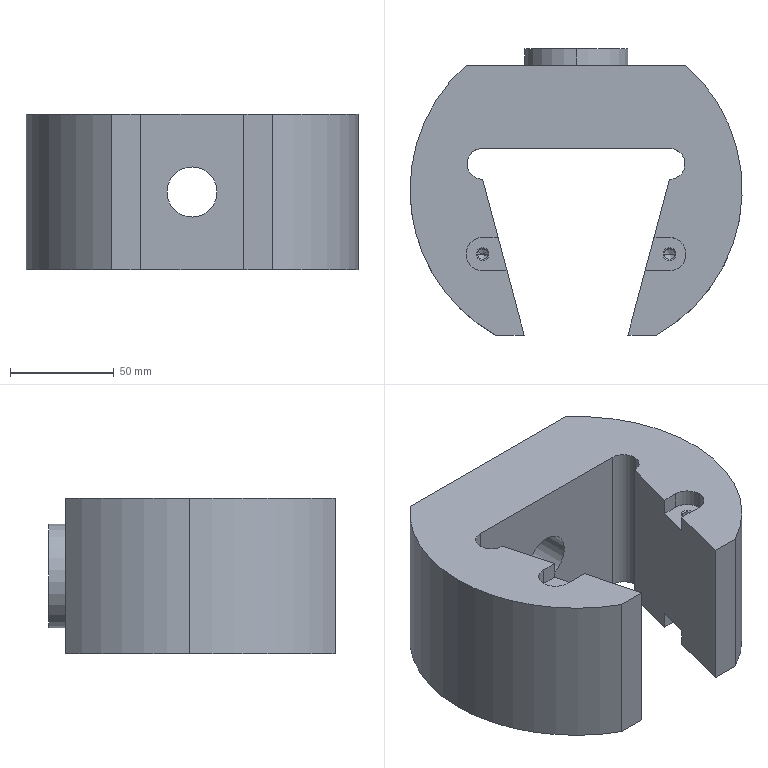Part | SolidWorks | features ICE 6, 3DProfileFeature 1, Extrusion 1, HoleWzd 1 | 1 solid | 61 faces | box 160 x 138 x 75 mm | volume 835946 mm3 | cylinder 24 | plane 21 | cone 16 | commonest cylinder face diameters 5 x8 16 x6 15 x3 160 x3 24.2 x2 50 x2